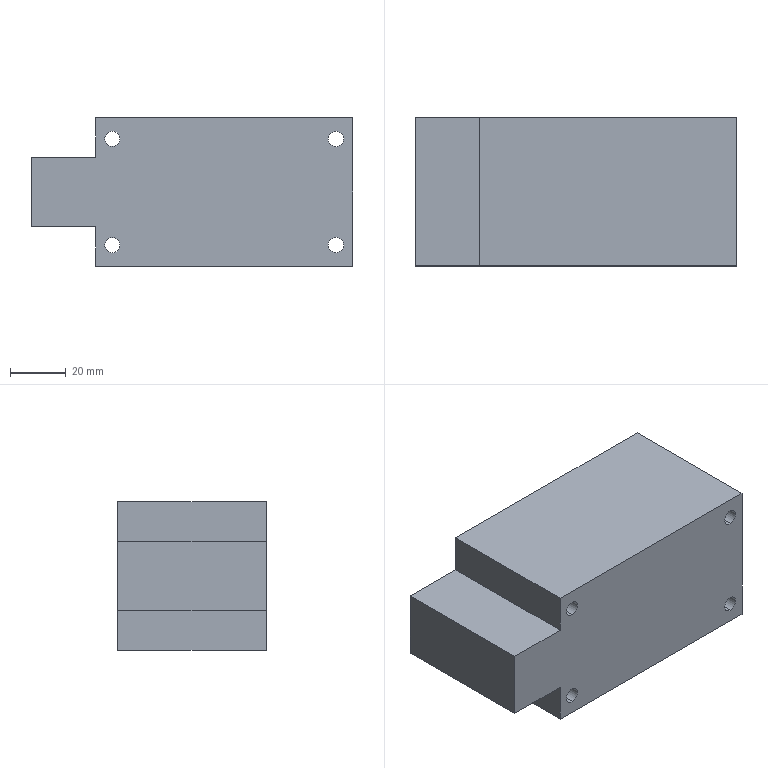Part | SolidWorks | features ICE 2, Extrusion 1 | 1 solid | 18 faces | box 115 x 53 x 53 mm | volume 283866 mm3 | plane 10 | cylinder 8 | commonest cylinder face diameters 5.5 x8
STEP:
#1=CARTESIAN_POINT('',(-28.5,0.,16.25));
#2=VERTEX_POINT('',#1);
#3=CARTESIAN_POINT('',(-28.5,0.,21.75));
#4=VERTEX_POINT('',#3);
#5=CARTESIAN_POINT('',(-28.5,0.,19.));
#6=DIRECTION('',(0.,1.,0.));
#7=DIRECTION('',(0.,0.,1.));
#8=AXIS2_PLACEMENT_3D('',#5,#6,#7);
#9=CIRCLE('',#8,2.75);
#10=EDGE_CURVE('',#2,#4,#9,.T.);
#11=ORIENTED_EDGE('',*,*,#10,.F.);
#12=CARTESIAN_POINT('',(-28.5,53.,16.25));
#13=VERTEX_POINT('',#12);
#14=CARTESIAN_POINT('',(-28.5,0.,16.25));
#15=DIRECTION('',(0.,1.,0.));
#16=VECTOR('',#15,1000.);
#17=LINE('',#14,#16);
#18=EDGE_CURVE('',#2,#13,#17,.T.);
#19=ORIENTED_EDGE('',*,*,#18,.T.);
#20=CARTESIAN_POINT('',(-28.5,53.,21.75));
#21=VERTEX_POINT('',#20);
#22=CARTESIAN_POINT('',(-28.5,53.,19.));
#23=DIRECTION('',(0.,1.,0.));
#24=DIRECTION('',(0.,0.,1.));
#25=AXIS2_PLACEMENT_3D('',#22,#23,#24);
#26=CIRCLE('',#25,2.75);
#27=EDGE_CURVE('',#13,#21,#26,.T.);
#28=ORIENTED_EDGE('',*,*,#27,.T.);
#29=CARTESIAN_POINT('',(-28.5,0.,21.75));
#30=DIRECTION('',(0.,1.,0.));
#31=VECTOR('',#30,1000.);
#32=LINE('',#29,#31);
#33=EDGE_CURVE('',#4,#21,#32,.T.);
#34=ORIENTED_EDGE('',*,*,#33,.F.);
#35=EDGE_LOOP('',(#11,#19,#28,#34));
#36=FACE_OUTER_BOUND('',#35,.T.);
#37=CARTESIAN_POINT('',(-28.5,0.,19.));
#38=DIRECTION('',(0.,1.,0.));
#39=DIRECTION('',(0.,0.,1.));
#40=AXIS2_PLACEMENT_3D('',#37,#38,#39);
#41=CYLINDRICAL_SURFACE('',#40,2.75);
#42=ADVANCED_FACE('',(#36),#41,.F.);
#43=CARTESIAN_POINT('',(51.5,0.,16.25));
#44=VERTEX_POINT('',#43);
#45=CARTESIAN_POINT('',(51.5,0.,21.75));
#46=VERTEX_POINT('',#45);
#47=CARTESIAN_POINT('',(51.5,0.,19.));
#48=DIRECTION('',(0.,1.,0.));
#49=DIRECTION('',(0.,0.,1.));
#50=AXIS2_PLACEMENT_3D('',#47,#48,#49);
#51=CIRCLE('',#50,2.75);
#52=EDGE_CURVE('',#44,#46,#51,.T.);
#53=ORIENTED_EDGE('',*,*,#52,.F.);
#54=CARTESIAN_POINT('',(51.5,53.,16.25));
#55=VERTEX_POINT('',#54);
#56=CARTESIAN_POINT('',(51.5,0.,16.25));
#57=DIRECTION('',(0.,1.,0.));
#58=VECTOR('',#57,1000.);
#59=LINE('',#56,#58);
#60=EDGE_CURVE('',#44,#55,#59,.T.);
#61=ORIENTED_EDGE('',*,*,#60,.T.);
#62=CARTESIAN_POINT('',(51.5,53.,21.75));
#63=VERTEX_POINT('',#62);
#64=CARTESIAN_POINT('',(51.5,53.,19.));
#65=DIRECTION('',(0.,1.,0.));
#66=DIRECTION('',(0.,0.,1.));
#67=AXIS2_PLACEMENT_3D('',#64,#65,#66);
#68=CIRCLE('',#67,2.75);
#69=EDGE_CURVE('',#55,#63,#68,.T.);
#70=ORIENTED_EDGE('',*,*,#69,.T.);
#71=CARTESIAN_POINT('',(51.5,0.,21.75));
#72=DIRECTION('',(0.,1.,0.));
#73=VECTOR('',#72,1000.);
#74=LINE('',#71,#73);
#75=EDGE_CURVE('',#46,#63,#74,.T.);
#76=ORIENTED_EDGE('',*,*,#75,.F.);
#77=EDGE_LOOP('',(#53,#61,#70,#76));
#78=FACE_OUTER_BOUND('',#77,.T.);
#79=CARTESIAN_POINT('',(51.5,0.,19.));
#80=DIRECTION('',(0.,1.,0.));
#81=DIRECTION('',(0.,0.,1.));
#82=AXIS2_PLACEMENT_3D('',#79,#80,#81);
#83=CYLINDRICAL_SURFACE('',#82,2.75);
#84=ADVANCED_FACE('',(#78),#83,.F.);
#85=CARTESIAN_POINT('',(51.5,0.,-21.75));
#86=VERTEX_POINT('',#85);
#87=CARTESIAN_POINT('',(51.5,0.,-16.25));
#88=VERTEX_POINT('',#87);
#89=CARTESIAN_POINT('',(51.5,0.,-19.));
#90=DIRECTION('',(0.,1.,0.));
#91=DIRECTION('',(0.,0.,1.));
#92=AXIS2_PLACEMENT_3D('',#89,#90,#91);
#93=CIRCLE('',#92,2.75);
#94=EDGE_CURVE('',#86,#88,#93,.T.);
#95=ORIENTED_EDGE('',*,*,#94,.F.);
#96=CARTESIAN_POINT('',(51.5,53.,-21.75));
#97=VERTEX_POINT('',#96);
#98=CARTESIAN_POINT('',(51.5,0.,-21.75));
#99=DIRECTION('',(0.,1.,0.));
#100=VECTOR('',#99,1000.);
#101=LINE('',#98,#100);
#102=EDGE_CURVE('',#86,#97,#101,.T.);
#103=ORIENTED_EDGE('',*,*,#102,.T.);
#104=CARTESIAN_POINT('',(51.5,53.,-16.25));
#105=VERTEX_POINT('',#104);
#106=CARTESIAN_POINT('',(51.5,53.,-19.));
#107=DIRECTION('',(0.,1.,0.));
#108=DIRECTION('',(0.,0.,1.));
#109=AXIS2_PLACEMENT_3D('',#106,#107,#108);
#110=CIRCLE('',#109,2.75);
#111=EDGE_CURVE('',#97,#105,#110,.T.);
#112=ORIENTED_EDGE('',*,*,#111,.T.);
#113=CARTESIAN_POINT('',(51.5,0.,-16.25));
#114=DIRECTION('',(0.,1.,0.));
#115=VECTOR('',#114,1000.);
#116=LINE('',#113,#115);
#117=EDGE_CURVE('',#88,#105,#116,.T.);
#118=ORIENTED_EDGE('',*,*,#117,.F.);
#119=EDGE_LOOP('',(#95,#103,#112,#118));
#120=FACE_OUTER_BOUND('',#119,.T.);
#121=CARTESIAN_POINT('',(51.5,0.,-19.));
#122=DIRECTION('',(0.,1.,0.));
#123=DIRECTION('',(0.,0.,1.));
#124=AXIS2_PLACEMENT_3D('',#121,#122,#123);
#125=CYLINDRICAL_SURFACE('',#124,2.75);
#126=ADVANCED_FACE('',(#120),#125,.F.);
#127=CARTESIAN_POINT('',(-28.5,0.,-21.75));
#128=VERTEX_POINT('',#127);
#129=CARTESIAN_POINT('',(-28.5,0.,-16.25));
#130=VERTEX_POINT('',#129);
#131=CARTESIAN_POINT('',(-28.5,0.,-19.));
#132=DIRECTION('',(0.,1.,0.));
#133=DIRECTION('',(0.,0.,1.));
#134=AXIS2_PLACEMENT_3D('',#131,#132,#133);
#135=CIRCLE('',#134,2.75);
#136=EDGE_CURVE('',#128,#130,#135,.T.);
#137=ORIENTED_EDGE('',*,*,#136,.F.);
#138=CARTESIAN_POINT('',(-28.5,53.,-21.75));
#139=VERTEX_POINT('',#138);
#140=CARTESIAN_POINT('',(-28.5,0.,-21.75));
#141=DIRECTION('',(0.,1.,0.));
#142=VECTOR('',#141,1000.);
#143=LINE('',#140,#142);
#144=EDGE_CURVE('',#128,#139,#143,.T.);
#145=ORIENTED_EDGE('',*,*,#144,.T.);
#146=CARTESIAN_POINT('',(-28.5,53.,-16.25));
#147=VERTEX_POINT('',#146);
#148=CARTESIAN_POINT('',(-28.5,53.,-19.));
#149=DIRECTION('',(0.,1.,0.));
#150=DIRECTION('',(0.,0.,1.));
#151=AXIS2_PLACEMENT_3D('',#148,#149,#150);
#152=CIRCLE('',#151,2.75);
#153=EDGE_CURVE('',#139,#147,#152,.T.);
#154=ORIENTED_EDGE('',*,*,#153,.T.);
#155=CARTESIAN_POINT('',(-28.5,0.,-16.25));
#156=DIRECTION('',(0.,1.,0.));
#157=VECTOR('',#156,1000.);
#158=LINE('',#155,#157);
#159=EDGE_CURVE('',#130,#147,#158,.T.);
#160=ORIENTED_EDGE('',*,*,#159,.F.);
#161=EDGE_LOOP('',(#137,#145,#154,#160));
#162=FACE_OUTER_BOUND('',#161,.T.);
#163=CARTESIAN_POINT('',(-28.5,0.,-19.));
#164=DIRECTION('',(0.,1.,0.));
#165=DIRECTION('',(0.,0.,1.));
#166=AXIS2_PLACEMENT_3D('',#163,#164,#165);
#167=CYLINDRICAL_SURFACE('',#166,2.75);
#168=ADVANCED_FACE('',(#162),#167,.F.);
#169=CARTESIAN_POINT('',(57.5,0.,26.5));
#170=VERTEX_POINT('',#169);
#171=CARTESIAN_POINT('',(57.5,0.,-26.5));
#172=VERTEX_POINT('',#171);
#173=CARTESIAN_POINT('',(57.5,0.,-26.5));
#174=DIRECTION('',(0.,0.,-1.));
#175=VECTOR('',#174,1000.);
#176=LINE('',#173,#175);
#177=EDGE_CURVE('',#170,#172,#176,.T.);
#178=ORIENTED_EDGE('',*,*,#177,.T.);
#179=CARTESIAN_POINT('',(57.5,53.,-26.5));
#180=VERTEX_POINT('',#179);
#181=CARTESIAN_POINT('',(57.5,53.,-26.5));
#182=DIRECTION('',(0.,-1.,0.));
#183=VECTOR('',#182,1000.);
#184=LINE('',#181,#183);
#185=EDGE_CURVE('',#180,#172,#184,.T.);
#186=ORIENTED_EDGE('',*,*,#185,.F.);
#187=CARTESIAN_POINT('',(57.5,53.,26.5));
#188=VERTEX_POINT('',#187);
#189=CARTESIAN_POINT('',(57.5,53.,-26.5));
#190=DIRECTION('',(0.,0.,-1.));
#191=VECTOR('',#190,1000.);
#192=LINE('',#189,#191);
#193=EDGE_CURVE('',#188,#180,#192,.T.);
#194=ORIENTED_EDGE('',*,*,#193,.F.);
#195=CARTESIAN_POINT('',(57.5,53.,26.5));
#196=DIRECTION('',(0.,-1.,0.));
#197=VECTOR('',#196,1000.);
#198=LINE('',#195,#197);
#199=EDGE_CURVE('',#188,#170,#198,.T.);
#200=ORIENTED_EDGE('',*,*,#199,.T.);
#201=EDGE_LOOP('',(#178,#186,#194,#200));
#202=FACE_OUTER_BOUND('',#201,.T.);
#203=CARTESIAN_POINT('',(57.5,53.,-26.5));
#204=DIRECTION('',(-1.,0.,0.));
#205=DIRECTION('',(0.,0.,1.));
#206=AXIS2_PLACEMENT_3D('',#203,#204,#205);
#207=PLANE('',#206);
#208=ADVANCED_FACE('',(#202),#207,.F.);
#209=CARTESIAN_POINT('',(-34.5,0.,-26.5));
#210=VERTEX_POINT('',#209);
#211=CARTESIAN_POINT('',(-57.5,0.,-26.5));
#212=DIRECTION('',(-1.,0.,0.));
#213=VECTOR('',#212,1000.);
#214=LINE('',#211,#213);
#215=EDGE_CURVE('',#172,#210,#214,.T.);
#216=ORIENTED_EDGE('',*,*,#215,.T.);
#217=CARTESIAN_POINT('',(-34.5,53.,-26.5));
#218=VERTEX_POINT('',#217);
#219=CARTESIAN_POINT('',(-34.5,53.,-26.5));
#220=DIRECTION('',(0.,1.,0.));
#221=VECTOR('',#220,1000.);
#222=LINE('',#219,#221);
#223=EDGE_CURVE('',#210,#218,#222,.T.);
#224=ORIENTED_EDGE('',*,*,#223,.T.);
#225=CARTESIAN_POINT('',(-57.5,53.,-26.5));
#226=DIRECTION('',(-1.,0.,0.));
#227=VECTOR('',#226,1000.);
#228=LINE('',#225,#227);
#229=EDGE_CURVE('',#180,#218,#228,.T.);
#230=ORIENTED_EDGE('',*,*,#229,.F.);
#231=ORIENTED_EDGE('',*,*,#185,.T.);
#232=EDGE_LOOP('',(#216,#224,#230,#231));
#233=FACE_OUTER_BOUND('',#232,.T.);
#234=CARTESIAN_POINT('',(-57.5,53.,-26.5));
#235=DIRECTION('',(0.,0.,1.));
#236=DIRECTION('',(1.,0.,0.));
#237=AXIS2_PLACEMENT_3D('',#234,#235,#236);
#238=PLANE('',#237);
#239=ADVANCED_FACE('',(#233),#238,.F.);
#240=CARTESIAN_POINT('',(-57.5,53.,-12.5));
#241=VERTEX_POINT('',#240);
#242=CARTESIAN_POINT('',(-57.5,53.,12.5));
#243=VERTEX_POINT('',#242);
#244=CARTESIAN_POINT('',(-57.5,53.,-26.5));
#245=DIRECTION('',(0.,0.,1.));
#246=VECTOR('',#245,1000.);
#247=LINE('',#244,#246);
#248=EDGE_CURVE('',#241,#243,#247,.T.);
#249=ORIENTED_EDGE('',*,*,#248,.F.);
#250=CARTESIAN_POINT('',(-57.5,0.,-12.5));
#251=VERTEX_POINT('',#250);
#252=CARTESIAN_POINT('',(-57.5,53.,-12.5));
#253=DIRECTION('',(0.,-1.,0.));
#254=VECTOR('',#253,1000.);
#255=LINE('',#252,#254);
#256=EDGE_CURVE('',#241,#251,#255,.T.);
#257=ORIENTED_EDGE('',*,*,#256,.T.);
#258=CARTESIAN_POINT('',(-57.5,0.,12.5));
#259=VERTEX_POINT('',#258);
#260=CARTESIAN_POINT('',(-57.5,0.,-26.5));
#261=DIRECTION('',(0.,0.,1.));
#262=VECTOR('',#261,1000.);
#263=LINE('',#260,#262);
#264=EDGE_CURVE('',#251,#259,#263,.T.);
#265=ORIENTED_EDGE('',*,*,#264,.T.);
#266=CARTESIAN_POINT('',(-57.5,53.,12.5));
#267=DIRECTION('',(0.,1.,0.));
#268=VECTOR('',#267,1000.);
#269=LINE('',#266,#268);
#270=EDGE_CURVE('',#259,#243,#269,.T.);
#271=ORIENTED_EDGE('',*,*,#270,.T.);
#272=EDGE_LOOP('',(#249,#257,#265,#271));
#273=FACE_OUTER_BOUND('',#272,.T.);
#274=CARTESIAN_POINT('',(-57.5,53.,-26.5));
#275=DIRECTION('',(1.,0.,0.));
#276=DIRECTION('',(0.,0.,-1.));
#277=AXIS2_PLACEMENT_3D('',#274,#275,#276);
#278=PLANE('',#277);
#279=ADVANCED_FACE('',(#273),#278,.F.);
#280=CARTESIAN_POINT('',(-34.5,53.,26.5));
#281=VERTEX_POINT('',#280);
#282=CARTESIAN_POINT('',(-57.5,53.,26.5));
#283=DIRECTION('',(1.,0.,0.));
#284=VECTOR('',#283,1000.);
#285=LINE('',#282,#284);
#286=EDGE_CURVE('',#281,#188,#285,.T.);
#287=ORIENTED_EDGE('',*,*,#286,.F.);
#288=CARTESIAN_POINT('',(-34.5,0.,26.5));
#289=VERTEX_POINT('',#288);
#290=CARTESIAN_POINT('',(-34.5,53.,26.5));
#291=DIRECTION('',(0.,-1.,0.));
#292=VECTOR('',#291,1000.);
#293=LINE('',#290,#292);
#294=EDGE_CURVE('',#281,#289,#293,.T.);
#295=ORIENTED_EDGE('',*,*,#294,.T.);
#296=CARTESIAN_POINT('',(-57.5,0.,26.5));
#297=DIRECTION('',(1.,0.,0.));
#298=VECTOR('',#297,1000.);
#299=LINE('',#296,#298);
#300=EDGE_CURVE('',#289,#170,#299,.T.);
#301=ORIENTED_EDGE('',*,*,#300,.T.);
#302=ORIENTED_EDGE('',*,*,#199,.F.);
#303=EDGE_LOOP('',(#287,#295,#301,#302));
#304=FACE_OUTER_BOUND('',#303,.T.);
#305=CARTESIAN_POINT('',(-57.5,53.,26.5));
#306=DIRECTION('',(0.,0.,-1.));
#307=DIRECTION('',(-1.,0.,0.));
#308=AXIS2_PLACEMENT_3D('',#305,#306,#307);
#309=PLANE('',#308);
#310=ADVANCED_FACE('',(#304),#309,.F.);
#311=CARTESIAN_POINT('',(-28.5,53.,19.));
#312=DIRECTION('',(0.,1.,0.));
#313=DIRECTION('',(0.,0.,1.));
#314=AXIS2_PLACEMENT_3D('',#311,#312,#313);
#315=CIRCLE('',#314,2.75);
#316=EDGE_CURVE('',#21,#13,#315,.T.);
#317=ORIENTED_EDGE('',*,*,#316,.F.);
#318=ORIENTED_EDGE('',*,*,#27,.F.);
#319=EDGE_LOOP('',(#317,#318));
#320=FACE_BOUND('',#319,.T.);
#321=CARTESIAN_POINT('',(51.5,53.,19.));
#322=DIRECTION('',(0.,1.,0.));
#323=DIRECTION('',(0.,0.,1.));
#324=AXIS2_PLACEMENT_3D('',#321,#322,#323);
#325=CIRCLE('',#324,2.75);
#326=EDGE_CURVE('',#63,#55,#325,.T.);
#327=ORIENTED_EDGE('',*,*,#326,.F.);
#328=ORIENTED_EDGE('',*,*,#69,.F.);
#329=EDGE_LOOP('',(#327,#328));
#330=FACE_BOUND('',#329,.T.);
#331=CARTESIAN_POINT('',(51.5,53.,-19.));
#332=DIRECTION('',(0.,1.,0.));
#333=DIRECTION('',(0.,0.,1.));
#334=AXIS2_PLACEMENT_3D('',#331,#332,#333);
#335=CIRCLE('',#334,2.75);
#336=EDGE_CURVE('',#105,#97,#335,.T.);
#337=ORIENTED_EDGE('',*,*,#336,.F.);
#338=ORIENTED_EDGE('',*,*,#111,.F.);
#339=EDGE_LOOP('',(#337,#338));
#340=FACE_BOUND('',#339,.T.);
#341=CARTESIAN_POINT('',(-28.5,53.,-19.));
#342=DIRECTION('',(0.,1.,0.));
#343=DIRECTION('',(0.,0.,1.));
#344=AXIS2_PLACEMENT_3D('',#341,#342,#343);
#345=CIRCLE('',#344,2.75);
#346=EDGE_CURVE('',#147,#139,#345,.T.);
#347=ORIENTED_EDGE('',*,*,#346,.F.);
#348=ORIENTED_EDGE('',*,*,#153,.F.);
#349=EDGE_LOOP('',(#347,#348));
#350=FACE_BOUND('',#349,.T.);
#351=CARTESIAN_POINT('',(-34.5,53.,-12.5));
#352=VERTEX_POINT('',#351);
#353=CARTESIAN_POINT('',(-34.5,53.,-40.5));
#354=DIRECTION('',(0.,0.,-1.));
#355=VECTOR('',#354,1000.);
#356=LINE('',#353,#355);
#357=EDGE_CURVE('',#352,#218,#356,.T.);
#358=ORIENTED_EDGE('',*,*,#357,.F.);
#359=CARTESIAN_POINT('',(-80.5,53.,-12.5));
#360=DIRECTION('',(1.,0.,0.));
#361=VECTOR('',#360,1000.);
#362=LINE('',#359,#361);
#363=EDGE_CURVE('',#241,#352,#362,.T.);
#364=ORIENTED_EDGE('',*,*,#363,.F.);
#365=ORIENTED_EDGE('',*,*,#248,.T.);
#366=CARTESIAN_POINT('',(-34.5,53.,12.5));
#367=VERTEX_POINT('',#366);
#368=CARTESIAN_POINT('',(-80.5,53.,12.5));
#369=DIRECTION('',(-1.,0.,0.));
#370=VECTOR('',#369,1000.);
#371=LINE('',#368,#370);
#372=EDGE_CURVE('',#367,#243,#371,.T.);
#373=ORIENTED_EDGE('',*,*,#372,.F.);
#374=CARTESIAN_POINT('',(-34.5,53.,40.5));
#375=DIRECTION('',(0.,0.,-1.));
#376=VECTOR('',#375,1000.);
#377=LINE('',#374,#376);
#378=EDGE_CURVE('',#281,#367,#377,.T.);
#379=ORIENTED_EDGE('',*,*,#378,.F.);
#380=ORIENTED_EDGE('',*,*,#286,.T.);
#381=ORIENTED_EDGE('',*,*,#193,.T.);
#382=ORIENTED_EDGE('',*,*,#229,.T.);
#383=EDGE_LOOP('',(#358,#364,#365,#373,#379,#380,#381,#382));
#384=FACE_OUTER_BOUND('',#383,.T.);
#385=CARTESIAN_POINT('',(0.,53.,0.));
#386=DIRECTION('',(0.,1.,0.));
#387=DIRECTION('',(0.,0.,1.));
#388=AXIS2_PLACEMENT_3D('',#385,#386,#387);
#389=PLANE('',#388);
#390=ADVANCED_FACE('',(#320,#330,#340,#350,#384),#389,.T.);
#391=CARTESIAN_POINT('',(-28.5,0.,19.));
#392=DIRECTION('',(0.,1.,0.));
#393=DIRECTION('',(0.,0.,1.));
#394=AXIS2_PLACEMENT_3D('',#391,#392,#393);
#395=CIRCLE('',#394,2.75);
#396=EDGE_CURVE('',#4,#2,#395,.T.);
#397=ORIENTED_EDGE('',*,*,#396,.T.);
#398=ORIENTED_EDGE('',*,*,#10,.T.);
#399=EDGE_LOOP('',(#397,#398));
#400=FACE_BOUND('',#399,.T.);
#401=CARTESIAN_POINT('',(51.5,0.,19.));
#402=DIRECTION('',(0.,1.,0.));
#403=DIRECTION('',(0.,0.,1.));
#404=AXIS2_PLACEMENT_3D('',#401,#402,#403);
#405=CIRCLE('',#404,2.75);
#406=EDGE_CURVE('',#46,#44,#405,.T.);
#407=ORIENTED_EDGE('',*,*,#406,.T.);
#408=ORIENTED_EDGE('',*,*,#52,.T.);
#409=EDGE_LOOP('',(#407,#408));
#410=FACE_BOUND('',#409,.T.);
#411=CARTESIAN_POINT('',(51.5,0.,-19.));
#412=DIRECTION('',(0.,1.,0.));
#413=DIRECTION('',(0.,0.,1.));
#414=AXIS2_PLACEMENT_3D('',#411,#412,#413);
#415=CIRCLE('',#414,2.75);
#416=EDGE_CURVE('',#88,#86,#415,.T.);
#417=ORIENTED_EDGE('',*,*,#416,.T.);
#418=ORIENTED_EDGE('',*,*,#94,.T.);
#419=EDGE_LOOP('',(#417,#418));
#420=FACE_BOUND('',#419,.T.);
#421=CARTESIAN_POINT('',(-28.5,0.,-19.));
#422=DIRECTION('',(0.,1.,0.));
#423=DIRECTION('',(0.,0.,1.));
#424=AXIS2_PLACEMENT_3D('',#421,#422,#423);
#425=CIRCLE('',#424,2.75);
#426=EDGE_CURVE('',#130,#128,#425,.T.);
#427=ORIENTED_EDGE('',*,*,#426,.T.);
#428=ORIENTED_EDGE('',*,*,#136,.T.);
#429=EDGE_LOOP('',(#427,#428));
#430=FACE_BOUND('',#429,.T.);
#431=CARTESIAN_POINT('',(-34.5,0.,-12.5));
#432=VERTEX_POINT('',#431);
#433=CARTESIAN_POINT('',(0.,0.,-12.5));
#434=DIRECTION('',(1.,0.,0.));
#435=VECTOR('',#434,1000.);
#436=LINE('',#433,#435);
#437=EDGE_CURVE('',#251,#432,#436,.T.);
#438=ORIENTED_EDGE('',*,*,#437,.T.);
#439=CARTESIAN_POINT('',(-34.5,0.,-40.5));
#440=DIRECTION('',(0.,0.,-1.));
#441=VECTOR('',#440,1000.);
#442=LINE('',#439,#441);
#443=EDGE_CURVE('',#432,#210,#442,.T.);
#444=ORIENTED_EDGE('',*,*,#443,.T.);
#445=ORIENTED_EDGE('',*,*,#215,.F.);
#446=ORIENTED_EDGE('',*,*,#177,.F.);
#447=ORIENTED_EDGE('',*,*,#300,.F.);
#448=CARTESIAN_POINT('',(-34.5,0.,12.5));
#449=VERTEX_POINT('',#448);
#450=CARTESIAN_POINT('',(-34.5,0.,0.));
#451=DIRECTION('',(0.,0.,-1.));
#452=VECTOR('',#451,1000.);
#453=LINE('',#450,#452);
#454=EDGE_CURVE('',#289,#449,#453,.T.);
#455=ORIENTED_EDGE('',*,*,#454,.T.);
#456=CARTESIAN_POINT('',(-80.5,0.,12.5));
#457=DIRECTION('',(-1.,0.,0.));
#458=VECTOR('',#457,1000.);
#459=LINE('',#456,#458);
#460=EDGE_CURVE('',#449,#259,#459,.T.);
#461=ORIENTED_EDGE('',*,*,#460,.T.);
#462=ORIENTED_EDGE('',*,*,#264,.F.);
#463=EDGE_LOOP('',(#438,#444,#445,#446,#447,#455,#461,#462));
#464=FACE_OUTER_BOUND('',#463,.T.);
#465=CARTESIAN_POINT('',(0.,0.,0.));
#466=DIRECTION('',(0.,1.,0.));
#467=DIRECTION('',(0.,0.,1.));
#468=AXIS2_PLACEMENT_3D('',#465,#466,#467);
#469=PLANE('',#468);
#470=ADVANCED_FACE('',(#400,#410,#420,#430,#464),#469,.F.);
#471=ORIENTED_EDGE('',*,*,#378,.T.);
#472=CARTESIAN_POINT('',(-34.5,0.,12.5));
#473=DIRECTION('',(0.,1.,0.));
#474=VECTOR('',#473,1000.);
#475=LINE('',#472,#474);
#476=EDGE_CURVE('',#449,#367,#475,.T.);
#477=ORIENTED_EDGE('',*,*,#476,.F.);
#478=ORIENTED_EDGE('',*,*,#454,.F.);
#479=ORIENTED_EDGE('',*,*,#294,.F.);
#480=EDGE_LOOP('',(#471,#477,#478,#479));
#481=FACE_OUTER_BOUND('',#480,.T.);
#482=CARTESIAN_POINT('',(-34.5,0.,40.5));
#483=DIRECTION('',(1.,0.,0.));
#484=DIRECTION('',(0.,0.,-1.));
#485=AXIS2_PLACEMENT_3D('',#482,#483,#484);
#486=PLANE('',#485);
#487=ADVANCED_FACE('',(#481),#486,.F.);
#488=ORIENTED_EDGE('',*,*,#460,.F.);
#489=ORIENTED_EDGE('',*,*,#476,.T.);
#490=ORIENTED_EDGE('',*,*,#372,.T.);
#491=ORIENTED_EDGE('',*,*,#270,.F.);
#492=EDGE_LOOP('',(#488,#489,#490,#491));
#493=FACE_OUTER_BOUND('',#492,.T.);
#494=CARTESIAN_POINT('',(-80.5,0.,12.5));
#495=DIRECTION('',(0.,0.,-1.));
#496=DIRECTION('',(-1.,0.,0.));
#497=AXIS2_PLACEMENT_3D('',#494,#495,#496);
#498=PLANE('',#497);
#499=ADVANCED_FACE('',(#493),#498,.F.);
#500=ORIENTED_EDGE('',*,*,#443,.F.);
#501=CARTESIAN_POINT('',(-34.5,0.,-12.5));
#502=DIRECTION('',(0.,1.,0.));
#503=VECTOR('',#502,1000.);
#504=LINE('',#501,#503);
#505=EDGE_CURVE('',#432,#352,#504,.T.);
#506=ORIENTED_EDGE('',*,*,#505,.T.);
#507=ORIENTED_EDGE('',*,*,#357,.T.);
#508=ORIENTED_EDGE('',*,*,#223,.F.);
#509=EDGE_LOOP('',(#500,#506,#507,#508));
#510=FACE_OUTER_BOUND('',#509,.T.);
#511=CARTESIAN_POINT('',(-34.5,0.,-40.5));
#512=DIRECTION('',(1.,0.,0.));
#513=DIRECTION('',(0.,0.,-1.));
#514=AXIS2_PLACEMENT_3D('',#511,#512,#513);
#515=PLANE('',#514);
#516=ADVANCED_FACE('',(#510),#515,.F.);
#517=ORIENTED_EDGE('',*,*,#363,.T.);
#518=ORIENTED_EDGE('',*,*,#505,.F.);
#519=ORIENTED_EDGE('',*,*,#437,.F.);
#520=ORIENTED_EDGE('',*,*,#256,.F.);
#521=EDGE_LOOP('',(#517,#518,#519,#520));
#522=FACE_OUTER_BOUND('',#521,.T.);
#523=CARTESIAN_POINT('',(-80.5,0.,-12.5));
#524=DIRECTION('',(0.,0.,1.));
#525=DIRECTION('',(1.,0.,0.));
#526=AXIS2_PLACEMENT_3D('',#523,#524,#525);
#527=PLANE('',#526);
#528=ADVANCED_FACE('',(#522),#527,.F.);
#529=ORIENTED_EDGE('',*,*,#144,.F.);
#530=ORIENTED_EDGE('',*,*,#426,.F.);
#531=ORIENTED_EDGE('',*,*,#159,.T.);
#532=ORIENTED_EDGE('',*,*,#346,.T.);
#533=EDGE_LOOP('',(#529,#530,#531,#532));
#534=FACE_OUTER_BOUND('',#533,.T.);
#535=CARTESIAN_POINT('',(-28.5,0.,-19.));
#536=DIRECTION('',(0.,1.,0.));
#537=DIRECTION('',(0.,0.,1.));
#538=AXIS2_PLACEMENT_3D('',#535,#536,#537);
#539=CYLINDRICAL_SURFACE('',#538,2.75);
#540=ADVANCED_FACE('',(#534),#539,.F.);
#541=ORIENTED_EDGE('',*,*,#102,.F.);
#542=ORIENTED_EDGE('',*,*,#416,.F.);
#543=ORIENTED_EDGE('',*,*,#117,.T.);
#544=ORIENTED_EDGE('',*,*,#336,.T.);
#545=EDGE_LOOP('',(#541,#542,#543,#544));
#546=FACE_OUTER_BOUND('',#545,.T.);
#547=CARTESIAN_POINT('',(51.5,0.,-19.));
#548=DIRECTION('',(0.,1.,0.));
#549=DIRECTION('',(0.,0.,1.));
#550=AXIS2_PLACEMENT_3D('',#547,#548,#549);
#551=CYLINDRICAL_SURFACE('',#550,2.75);
#552=ADVANCED_FACE('',(#546),#551,.F.);
#553=ORIENTED_EDGE('',*,*,#60,.F.);
#554=ORIENTED_EDGE('',*,*,#406,.F.);
#555=ORIENTED_EDGE('',*,*,#75,.T.);
#556=ORIENTED_EDGE('',*,*,#326,.T.);
#557=EDGE_LOOP('',(#553,#554,#555,#556));
#558=FACE_OUTER_BOUND('',#557,.T.);
#559=CARTESIAN_POINT('',(51.5,0.,19.));
#560=DIRECTION('',(0.,1.,0.));
#561=DIRECTION('',(0.,0.,1.));
#562=AXIS2_PLACEMENT_3D('',#559,#560,#561);
#563=CYLINDRICAL_SURFACE('',#562,2.75);
#564=ADVANCED_FACE('',(#558),#563,.F.);
#565=ORIENTED_EDGE('',*,*,#18,.F.);
#566=ORIENTED_EDGE('',*,*,#396,.F.);
#567=ORIENTED_EDGE('',*,*,#33,.T.);
#568=ORIENTED_EDGE('',*,*,#316,.T.);
#569=EDGE_LOOP('',(#565,#566,#567,#568));
#570=FACE_OUTER_BOUND('',#569,.T.);
#571=CARTESIAN_POINT('',(-28.5,0.,19.));
#572=DIRECTION('',(0.,1.,0.));
#573=DIRECTION('',(0.,0.,1.));
#574=AXIS2_PLACEMENT_3D('',#571,#572,#573);
#575=CYLINDRICAL_SURFACE('',#574,2.75);
#576=ADVANCED_FACE('',(#570),#575,.F.);
#577=CLOSED_SHELL('',(#42,#84,#126,#168,#208,#239,#279,#310,#390,#470,#487,#499,#516,#528,#540,#552,#564,#576));
#578=MANIFOLD_SOLID_BREP('',#577);
#579=CARTESIAN_POINT('',(0.,0.,0.));
#580=DIRECTION('',(0.,0.,1.));
#581=DIRECTION('',(1.,0.,0.));
#582=AXIS2_PLACEMENT_3D('',#579,#580,#581);
#583=(LENGTH_UNIT()NAMED_UNIT(*)SI_UNIT(.MILLI.,.METRE.));
#584=UNCERTAINTY_MEASURE_WITH_UNIT(LENGTH_MEASURE(0.00001),#583,'','');
#585=(NAMED_UNIT(*)PLANE_ANGLE_UNIT()SI_UNIT($,.RADIAN.));
#586=(NAMED_UNIT(*)SI_UNIT($,.STERADIAN.)SOLID_ANGLE_UNIT());
#587=(GEOMETRIC_REPRESENTATION_CONTEXT(3)GLOBAL_UNCERTAINTY_ASSIGNED_CONTEXT((#584))GLOBAL_UNIT_ASSIGNED_CONTEXT((#583,#585,#586))REPRESENTATION_CONTEXT('',''));
#588=ADVANCED_BREP_SHAPE_REPRESENTATION('',(#578,#582),#587);